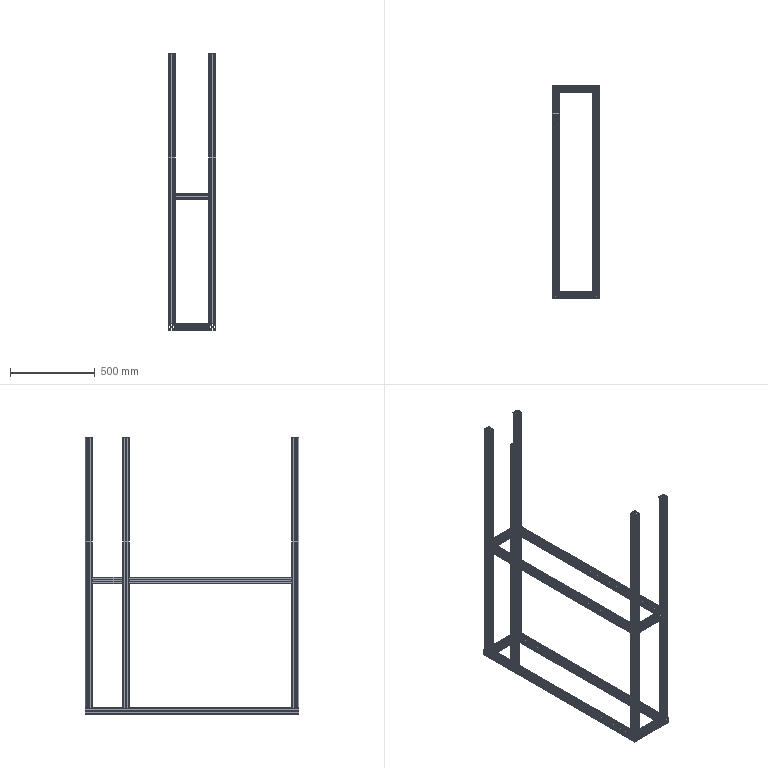Part | SolidWorks | features WeldCornerFeat 18, WeldMemberFeat 9, 3DProfileFeature 2, ICE 1, WeldmentFeature 1 | 14 solids | 1456 faces | box 280 x 1260 x 1635 mm | volume 6460308 mm3 | plane 1316 | cylinder 140 | commonest cylinder face diameters 5 x56 9 x56 6.8 x28